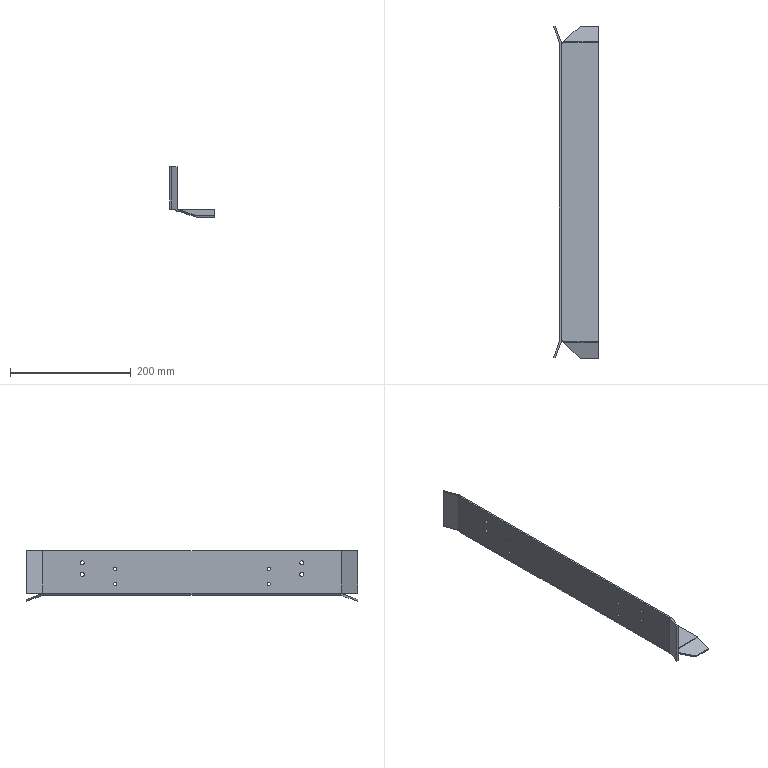Part | STEP file | IN-01-08-01-01_1 | 1 solid | 64 faces | box 74.017 x 548.705 x 83.447 mm | volume 217025 mm3 | plane 28 | cone 18 | cylinder 14 | spline 4 | commonest cylinder face diameters 2 x7 8 x7